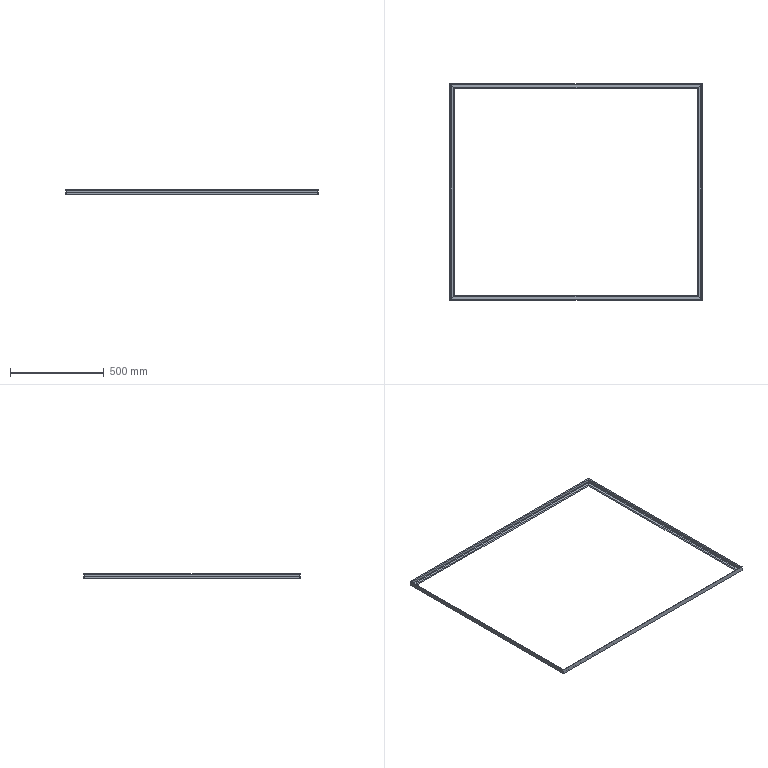Part | SolidWorks | features WeldMemberFeat 1, WeldmentFeature 1 | 4 solids | 36 faces | box 1348 x 1158 x 25 mm | volume 890268 mm3 | plane 24 | cylinder 12 | commonest cylinder face diameters 8 x8 7 x4
STEP:
#1=CARTESIAN_POINT('',(-649.,554.,0.));
#2=VERTEX_POINT('',#1);
#3=CARTESIAN_POINT('',(-674.,579.,0.));
#4=VERTEX_POINT('',#3);
#5=CARTESIAN_POINT('',(-82.5,-12.5,0.));
#6=DIRECTION('',(-0.7071,0.7071,0.));
#7=VECTOR('',#6,1000.);
#8=LINE('',#5,#7);
#9=EDGE_CURVE('',#2,#4,#8,.T.);
#10=ORIENTED_EDGE('',*,*,#9,.F.);
#11=CARTESIAN_POINT('',(-649.,-554.,0.));
#12=VERTEX_POINT('',#11);
#13=CARTESIAN_POINT('',(-649.,-579.,0.));
#14=DIRECTION('',(0.,1.,0.));
#15=VECTOR('',#14,1000.);
#16=LINE('',#13,#15);
#17=EDGE_CURVE('',#12,#2,#16,.T.);
#18=ORIENTED_EDGE('',*,*,#17,.F.);
#19=CARTESIAN_POINT('',(-674.,-579.,0.));
#20=VERTEX_POINT('',#19);
#21=CARTESIAN_POINT('',(-661.5,-566.5,0.));
#22=DIRECTION('',(0.7071,0.7071,0.));
#23=VECTOR('',#22,1000.);
#24=LINE('',#21,#23);
#25=EDGE_CURVE('',#20,#12,#24,.T.);
#26=ORIENTED_EDGE('',*,*,#25,.F.);
#27=CARTESIAN_POINT('',(-674.,-579.,0.));
#28=DIRECTION('',(0.,1.,0.));
#29=VECTOR('',#28,1000.);
#30=LINE('',#27,#29);
#31=EDGE_CURVE('',#20,#4,#30,.T.);
#32=ORIENTED_EDGE('',*,*,#31,.T.);
#33=EDGE_LOOP('',(#10,#18,#26,#32));
#34=FACE_OUTER_BOUND('',#33,.T.);
#35=CARTESIAN_POINT('',(-649.,-579.,0.));
#36=DIRECTION('',(0.,0.,1.));
#37=DIRECTION('',(1.,0.,0.));
#38=AXIS2_PLACEMENT_3D('',#35,#36,#37);
#39=PLANE('',#38);
#40=ADVANCED_FACE('',(#34),#39,.F.);
#41=CARTESIAN_POINT('',(-653.,558.,4.));
#42=VERTEX_POINT('',#41);
#43=CARTESIAN_POINT('',(-653.,558.,4.));
#44=CARTESIAN_POINT('',(-650.657,555.657,4.));
#45=CARTESIAN_POINT('',(-649.,554.,2.343));
#46=CARTESIAN_POINT('',(-649.,554.,0.));
#47=(BOUNDED_CURVE()B_SPLINE_CURVE(3,(#43,#44,#45,#46),.UNSPECIFIED.,.F.,.F.)B_SPLINE_CURVE_WITH_KNOTS((4,4),(1.571,3.142),.UNSPECIFIED.)CURVE()GEOMETRIC_REPRESENTATION_ITEM()RATIONAL_B_SPLINE_CURVE((1.,0.8047,0.8047,1.))REPRESENTATION_ITEM(''));
#48=EDGE_CURVE('',#42,#2,#47,.T.);
#49=ORIENTED_EDGE('',*,*,#48,.F.);
#50=CARTESIAN_POINT('',(-653.,-558.,4.));
#51=VERTEX_POINT('',#50);
#52=CARTESIAN_POINT('',(-653.,-579.,4.));
#53=DIRECTION('',(0.,1.,0.));
#54=VECTOR('',#53,1000.);
#55=LINE('',#52,#54);
#56=EDGE_CURVE('',#51,#42,#55,.T.);
#57=ORIENTED_EDGE('',*,*,#56,.F.);
#58=CARTESIAN_POINT('',(-649.,-554.,0.));
#59=CARTESIAN_POINT('',(-649.,-554.,2.343));
#60=CARTESIAN_POINT('',(-650.657,-555.657,4.));
#61=CARTESIAN_POINT('',(-653.,-558.,4.));
#62=(BOUNDED_CURVE()B_SPLINE_CURVE(3,(#58,#59,#60,#61),.UNSPECIFIED.,.F.,.F.)B_SPLINE_CURVE_WITH_KNOTS((4,4),(0.,1.571),.UNSPECIFIED.)CURVE()GEOMETRIC_REPRESENTATION_ITEM()RATIONAL_B_SPLINE_CURVE((1.,0.8047,0.8047,1.))REPRESENTATION_ITEM(''));
#63=EDGE_CURVE('',#12,#51,#62,.T.);
#64=ORIENTED_EDGE('',*,*,#63,.F.);
#65=ORIENTED_EDGE('',*,*,#17,.T.);
#66=EDGE_LOOP('',(#49,#57,#64,#65));
#67=FACE_OUTER_BOUND('',#66,.T.);
#68=CARTESIAN_POINT('',(-653.,-579.,0.));
#69=DIRECTION('',(0.,1.,0.));
#70=DIRECTION('',(0.,0.,1.));
#71=AXIS2_PLACEMENT_3D('',#68,#69,#70);
#72=CYLINDRICAL_SURFACE('',#71,4.);
#73=ADVANCED_FACE('',(#67),#72,.T.);
#74=CARTESIAN_POINT('',(-666.5,571.5,4.));
#75=VERTEX_POINT('',#74);
#76=CARTESIAN_POINT('',(-91.25,-3.75,4.));
#77=DIRECTION('',(0.7071,-0.7071,0.));
#78=VECTOR('',#77,1000.);
#79=LINE('',#76,#78);
#80=EDGE_CURVE('',#75,#42,#79,.T.);
#81=ORIENTED_EDGE('',*,*,#80,.F.);
#82=CARTESIAN_POINT('',(-666.5,-571.5,4.));
#83=VERTEX_POINT('',#82);
#84=CARTESIAN_POINT('',(-666.5,-579.,4.));
#85=DIRECTION('',(0.,1.,0.));
#86=VECTOR('',#85,1000.);
#87=LINE('',#84,#86);
#88=EDGE_CURVE('',#83,#75,#87,.T.);
#89=ORIENTED_EDGE('',*,*,#88,.F.);
#90=CARTESIAN_POINT('',(-670.25,-575.25,4.));
#91=DIRECTION('',(-0.7071,-0.7071,0.));
#92=VECTOR('',#91,1000.);
#93=LINE('',#90,#92);
#94=EDGE_CURVE('',#51,#83,#93,.T.);
#95=ORIENTED_EDGE('',*,*,#94,.F.);
#96=ORIENTED_EDGE('',*,*,#56,.T.);
#97=EDGE_LOOP('',(#81,#89,#95,#96));
#98=FACE_OUTER_BOUND('',#97,.T.);
#99=CARTESIAN_POINT('',(-666.5,-579.,4.));
#100=DIRECTION('',(0.,0.,-1.));
#101=DIRECTION('',(-1.,0.,0.));
#102=AXIS2_PLACEMENT_3D('',#99,#100,#101);
#103=PLANE('',#102);
#104=ADVANCED_FACE('',(#98),#103,.F.);
#105=CARTESIAN_POINT('',(-670.,575.,7.5));
#106=VERTEX_POINT('',#105);
#107=CARTESIAN_POINT('',(-670.,575.,7.5));
#108=CARTESIAN_POINT('',(-670.,575.,5.45));
#109=CARTESIAN_POINT('',(-668.55,573.55,4.));
#110=CARTESIAN_POINT('',(-666.5,571.5,4.));
#111=(BOUNDED_CURVE()B_SPLINE_CURVE(3,(#107,#108,#109,#110),.UNSPECIFIED.,.F.,.F.)B_SPLINE_CURVE_WITH_KNOTS((4,4),(0.,1.571),.UNSPECIFIED.)CURVE()GEOMETRIC_REPRESENTATION_ITEM()RATIONAL_B_SPLINE_CURVE((1.,0.8047,0.8047,1.))REPRESENTATION_ITEM(''));
#112=EDGE_CURVE('',#106,#75,#111,.T.);
#113=ORIENTED_EDGE('',*,*,#112,.F.);
#114=CARTESIAN_POINT('',(-670.,-575.,7.5));
#115=VERTEX_POINT('',#114);
#116=CARTESIAN_POINT('',(-670.,-579.,7.5));
#117=DIRECTION('',(0.,1.,0.));
#118=VECTOR('',#117,1000.);
#119=LINE('',#116,#118);
#120=EDGE_CURVE('',#115,#106,#119,.T.);
#121=ORIENTED_EDGE('',*,*,#120,.F.);
#122=CARTESIAN_POINT('',(-666.5,-571.5,4.));
#123=CARTESIAN_POINT('',(-668.55,-573.55,4.));
#124=CARTESIAN_POINT('',(-670.,-575.,5.45));
#125=CARTESIAN_POINT('',(-670.,-575.,7.5));
#126=(BOUNDED_CURVE()B_SPLINE_CURVE(3,(#122,#123,#124,#125),.UNSPECIFIED.,.F.,.F.)B_SPLINE_CURVE_WITH_KNOTS((4,4),(1.571,3.142),.UNSPECIFIED.)CURVE()GEOMETRIC_REPRESENTATION_ITEM()RATIONAL_B_SPLINE_CURVE((1.,0.8047,0.8047,1.))REPRESENTATION_ITEM(''));
#127=EDGE_CURVE('',#83,#115,#126,.T.);
#128=ORIENTED_EDGE('',*,*,#127,.F.);
#129=ORIENTED_EDGE('',*,*,#88,.T.);
#130=EDGE_LOOP('',(#113,#121,#128,#129));
#131=FACE_OUTER_BOUND('',#130,.T.);
#132=CARTESIAN_POINT('',(-666.5,-579.,7.5));
#133=DIRECTION('',(0.,1.,0.));
#134=DIRECTION('',(0.,0.,1.));
#135=AXIS2_PLACEMENT_3D('',#132,#133,#134);
#136=CYLINDRICAL_SURFACE('',#135,3.5);
#137=ADVANCED_FACE('',(#131),#136,.F.);
#138=CARTESIAN_POINT('',(-670.,575.,21.));
#139=VERTEX_POINT('',#138);
#140=CARTESIAN_POINT('',(-670.,575.,21.));
#141=DIRECTION('',(0.,0.,-1.));
#142=VECTOR('',#141,1000.);
#143=LINE('',#140,#142);
#144=EDGE_CURVE('',#139,#106,#143,.T.);
#145=ORIENTED_EDGE('',*,*,#144,.F.);
#146=CARTESIAN_POINT('',(-670.,-575.,21.));
#147=VERTEX_POINT('',#146);
#148=CARTESIAN_POINT('',(-670.,-579.,21.));
#149=DIRECTION('',(0.,1.,0.));
#150=VECTOR('',#149,1000.);
#151=LINE('',#148,#150);
#152=EDGE_CURVE('',#147,#139,#151,.T.);
#153=ORIENTED_EDGE('',*,*,#152,.F.);
#154=CARTESIAN_POINT('',(-670.,-575.,21.));
#155=DIRECTION('',(0.,0.,1.));
#156=VECTOR('',#155,1000.);
#157=LINE('',#154,#156);
#158=EDGE_CURVE('',#115,#147,#157,.T.);
#159=ORIENTED_EDGE('',*,*,#158,.F.);
#160=ORIENTED_EDGE('',*,*,#120,.T.);
#161=EDGE_LOOP('',(#145,#153,#159,#160));
#162=FACE_OUTER_BOUND('',#161,.T.);
#163=CARTESIAN_POINT('',(-670.,-579.,21.));
#164=DIRECTION('',(-1.,0.,0.));
#165=DIRECTION('',(0.,0.,1.));
#166=AXIS2_PLACEMENT_3D('',#163,#164,#165);
#167=PLANE('',#166);
#168=ADVANCED_FACE('',(#162),#167,.F.);
#169=CARTESIAN_POINT('',(-674.,579.,25.));
#170=VERTEX_POINT('',#169);
#171=CARTESIAN_POINT('',(-674.,579.,25.));
#172=CARTESIAN_POINT('',(-671.657,576.657,25.));
#173=CARTESIAN_POINT('',(-670.,575.,23.343));
#174=CARTESIAN_POINT('',(-670.,575.,21.));
#175=(BOUNDED_CURVE()B_SPLINE_CURVE(3,(#171,#172,#173,#174),.UNSPECIFIED.,.F.,.F.)B_SPLINE_CURVE_WITH_KNOTS((4,4),(1.571,3.142),.UNSPECIFIED.)CURVE()GEOMETRIC_REPRESENTATION_ITEM()RATIONAL_B_SPLINE_CURVE((1.,0.8047,0.8047,1.))REPRESENTATION_ITEM(''));
#176=EDGE_CURVE('',#170,#139,#175,.T.);
#177=ORIENTED_EDGE('',*,*,#176,.F.);
#178=CARTESIAN_POINT('',(-674.,-579.,25.));
#179=VERTEX_POINT('',#178);
#180=CARTESIAN_POINT('',(-674.,-579.,25.));
#181=DIRECTION('',(0.,1.,0.));
#182=VECTOR('',#181,1000.);
#183=LINE('',#180,#182);
#184=EDGE_CURVE('',#179,#170,#183,.T.);
#185=ORIENTED_EDGE('',*,*,#184,.F.);
#186=CARTESIAN_POINT('',(-670.,-575.,21.));
#187=CARTESIAN_POINT('',(-670.,-575.,23.343));
#188=CARTESIAN_POINT('',(-671.657,-576.657,25.));
#189=CARTESIAN_POINT('',(-674.,-579.,25.));
#190=(BOUNDED_CURVE()B_SPLINE_CURVE(3,(#186,#187,#188,#189),.UNSPECIFIED.,.F.,.F.)B_SPLINE_CURVE_WITH_KNOTS((4,4),(0.,1.571),.UNSPECIFIED.)CURVE()GEOMETRIC_REPRESENTATION_ITEM()RATIONAL_B_SPLINE_CURVE((1.,0.8047,0.8047,1.))REPRESENTATION_ITEM(''));
#191=EDGE_CURVE('',#147,#179,#190,.T.);
#192=ORIENTED_EDGE('',*,*,#191,.F.);
#193=ORIENTED_EDGE('',*,*,#152,.T.);
#194=EDGE_LOOP('',(#177,#185,#192,#193));
#195=FACE_OUTER_BOUND('',#194,.T.);
#196=CARTESIAN_POINT('',(-674.,-579.,21.));
#197=DIRECTION('',(0.,1.,0.));
#198=DIRECTION('',(0.,0.,1.));
#199=AXIS2_PLACEMENT_3D('',#196,#197,#198);
#200=CYLINDRICAL_SURFACE('',#199,4.);
#201=ADVANCED_FACE('',(#195),#200,.T.);
#202=CARTESIAN_POINT('',(-674.,579.,0.));
#203=DIRECTION('',(0.,0.,1.));
#204=VECTOR('',#203,1000.);
#205=LINE('',#202,#204);
#206=EDGE_CURVE('',#4,#170,#205,.T.);
#207=ORIENTED_EDGE('',*,*,#206,.F.);
#208=ORIENTED_EDGE('',*,*,#31,.F.);
#209=CARTESIAN_POINT('',(-674.,-579.,0.));
#210=DIRECTION('',(0.,0.,-1.));
#211=VECTOR('',#210,1000.);
#212=LINE('',#209,#211);
#213=EDGE_CURVE('',#179,#20,#212,.T.);
#214=ORIENTED_EDGE('',*,*,#213,.F.);
#215=ORIENTED_EDGE('',*,*,#184,.T.);
#216=EDGE_LOOP('',(#207,#208,#214,#215));
#217=FACE_OUTER_BOUND('',#216,.T.);
#218=CARTESIAN_POINT('',(-674.,-579.,0.));
#219=DIRECTION('',(1.,0.,0.));
#220=DIRECTION('',(0.,0.,-1.));
#221=AXIS2_PLACEMENT_3D('',#218,#219,#220);
#222=PLANE('',#221);
#223=ADVANCED_FACE('',(#217),#222,.F.);
#224=ORIENTED_EDGE('',*,*,#213,.T.);
#225=ORIENTED_EDGE('',*,*,#25,.T.);
#226=ORIENTED_EDGE('',*,*,#63,.T.);
#227=ORIENTED_EDGE('',*,*,#94,.T.);
#228=ORIENTED_EDGE('',*,*,#127,.T.);
#229=ORIENTED_EDGE('',*,*,#158,.T.);
#230=ORIENTED_EDGE('',*,*,#191,.T.);
#231=EDGE_LOOP('',(#224,#225,#226,#227,#228,#229,#230));
#232=FACE_OUTER_BOUND('',#231,.T.);
#233=CARTESIAN_POINT('',(-674.,-579.,0.));
#234=DIRECTION('',(0.7071,-0.7071,0.));
#235=DIRECTION('',(0.7071,0.7071,0.));
#236=AXIS2_PLACEMENT_3D('',#233,#234,#235);
#237=PLANE('',#236);
#238=ADVANCED_FACE('',(#232),#237,.T.);
#239=ORIENTED_EDGE('',*,*,#48,.T.);
#240=ORIENTED_EDGE('',*,*,#9,.T.);
#241=ORIENTED_EDGE('',*,*,#206,.T.);
#242=ORIENTED_EDGE('',*,*,#176,.T.);
#243=ORIENTED_EDGE('',*,*,#144,.T.);
#244=ORIENTED_EDGE('',*,*,#112,.T.);
#245=ORIENTED_EDGE('',*,*,#80,.T.);
#246=EDGE_LOOP('',(#239,#240,#241,#242,#243,#244,#245));
#247=FACE_OUTER_BOUND('',#246,.T.);
#248=CARTESIAN_POINT('',(-674.,579.,0.));
#249=DIRECTION('',(0.7071,0.7071,0.));
#250=DIRECTION('',(-0.7071,0.7071,0.));
#251=AXIS2_PLACEMENT_3D('',#248,#249,#250);
#252=PLANE('',#251);
#253=ADVANCED_FACE('',(#247),#252,.T.);
#254=CLOSED_SHELL('',(#40,#73,#104,#137,#168,#201,#223,#238,#253));
#255=MANIFOLD_SOLID_BREP('',#254);
#256=CARTESIAN_POINT('',(-649.,-554.,0.));
#257=VERTEX_POINT('',#256);
#258=CARTESIAN_POINT('',(-674.,-579.,0.));
#259=VERTEX_POINT('',#258);
#260=CARTESIAN_POINT('',(12.5,107.5,0.));
#261=DIRECTION('',(-0.7071,-0.7071,0.));
#262=VECTOR('',#261,1000.);
#263=LINE('',#260,#262);
#264=EDGE_CURVE('',#257,#259,#263,.T.);
#265=ORIENTED_EDGE('',*,*,#264,.F.);
#266=CARTESIAN_POINT('',(649.,-554.,0.));
#267=VERTEX_POINT('',#266);
#268=CARTESIAN_POINT('',(674.,-554.,0.));
#269=DIRECTION('',(-1.,0.,0.));
#270=VECTOR('',#269,1000.);
#271=LINE('',#268,#270);
#272=EDGE_CURVE('',#267,#257,#271,.T.);
#273=ORIENTED_EDGE('',*,*,#272,.F.);
#274=CARTESIAN_POINT('',(674.,-579.,0.));
#275=VERTEX_POINT('',#274);
#276=CARTESIAN_POINT('',(661.5,-566.5,0.));
#277=DIRECTION('',(-0.7071,0.7071,0.));
#278=VECTOR('',#277,1000.);
#279=LINE('',#276,#278);
#280=EDGE_CURVE('',#275,#267,#279,.T.);
#281=ORIENTED_EDGE('',*,*,#280,.F.);
#282=CARTESIAN_POINT('',(674.,-579.,0.));
#283=DIRECTION('',(-1.,0.,0.));
#284=VECTOR('',#283,1000.);
#285=LINE('',#282,#284);
#286=EDGE_CURVE('',#275,#259,#285,.T.);
#287=ORIENTED_EDGE('',*,*,#286,.T.);
#288=EDGE_LOOP('',(#265,#273,#281,#287));
#289=FACE_OUTER_BOUND('',#288,.T.);
#290=CARTESIAN_POINT('',(674.,-554.,0.));
#291=DIRECTION('',(0.,0.,1.));
#292=DIRECTION('',(1.,0.,0.));
#293=AXIS2_PLACEMENT_3D('',#290,#291,#292);
#294=PLANE('',#293);
#295=ADVANCED_FACE('',(#289),#294,.F.);
#296=CARTESIAN_POINT('',(-653.,-558.,4.));
#297=VERTEX_POINT('',#296);
#298=CARTESIAN_POINT('',(-653.,-558.,4.));
#299=CARTESIAN_POINT('',(-650.657,-555.657,4.));
#300=CARTESIAN_POINT('',(-649.,-554.,2.343));
#301=CARTESIAN_POINT('',(-649.,-554.,0.));
#302=(BOUNDED_CURVE()B_SPLINE_CURVE(3,(#298,#299,#300,#301),.UNSPECIFIED.,.F.,.T.)B_SPLINE_CURVE_WITH_KNOTS((4,4),(1.571,3.142),.UNSPECIFIED.)CURVE()GEOMETRIC_REPRESENTATION_ITEM()RATIONAL_B_SPLINE_CURVE((1.,0.8047,0.8047,1.))REPRESENTATION_ITEM(''));
#303=EDGE_CURVE('',#297,#257,#302,.T.);
#304=ORIENTED_EDGE('',*,*,#303,.F.);
#305=CARTESIAN_POINT('',(653.,-558.,4.));
#306=VERTEX_POINT('',#305);
#307=CARTESIAN_POINT('',(674.,-558.,4.));
#308=DIRECTION('',(-1.,0.,0.));
#309=VECTOR('',#308,1000.);
#310=LINE('',#307,#309);
#311=EDGE_CURVE('',#306,#297,#310,.T.);
#312=ORIENTED_EDGE('',*,*,#311,.F.);
#313=CARTESIAN_POINT('',(649.,-554.,0.));
#314=CARTESIAN_POINT('',(649.,-554.,2.343));
#315=CARTESIAN_POINT('',(650.657,-555.657,4.));
#316=CARTESIAN_POINT('',(653.,-558.,4.));
#317=(BOUNDED_CURVE()B_SPLINE_CURVE(3,(#313,#314,#315,#316),.UNSPECIFIED.,.F.,.F.)B_SPLINE_CURVE_WITH_KNOTS((4,4),(0.,1.571),.UNSPECIFIED.)CURVE()GEOMETRIC_REPRESENTATION_ITEM()RATIONAL_B_SPLINE_CURVE((1.,0.8047,0.8047,1.))REPRESENTATION_ITEM(''));
#318=EDGE_CURVE('',#267,#306,#317,.T.);
#319=ORIENTED_EDGE('',*,*,#318,.F.);
#320=ORIENTED_EDGE('',*,*,#272,.T.);
#321=EDGE_LOOP('',(#304,#312,#319,#320));
#322=FACE_OUTER_BOUND('',#321,.T.);
#323=CARTESIAN_POINT('',(674.,-558.,0.));
#324=DIRECTION('',(-1.,0.,0.));
#325=DIRECTION('',(0.,0.,1.));
#326=AXIS2_PLACEMENT_3D('',#323,#324,#325);
#327=CYLINDRICAL_SURFACE('',#326,4.);
#328=ADVANCED_FACE('',(#322),#327,.T.);
#329=CARTESIAN_POINT('',(-666.5,-571.5,4.));
#330=VERTEX_POINT('',#329);
#331=CARTESIAN_POINT('',(3.75,98.75,4.));
#332=DIRECTION('',(0.7071,0.7071,0.));
#333=VECTOR('',#332,1000.);
#334=LINE('',#331,#333);
#335=EDGE_CURVE('',#330,#297,#334,.T.);
#336=ORIENTED_EDGE('',*,*,#335,.F.);
#337=CARTESIAN_POINT('',(666.5,-571.5,4.));
#338=VERTEX_POINT('',#337);
#339=CARTESIAN_POINT('',(674.,-571.5,4.));
#340=DIRECTION('',(-1.,0.,0.));
#341=VECTOR('',#340,1000.);
#342=LINE('',#339,#341);
#343=EDGE_CURVE('',#338,#330,#342,.T.);
#344=ORIENTED_EDGE('',*,*,#343,.F.);
#345=CARTESIAN_POINT('',(670.25,-575.25,4.));
#346=DIRECTION('',(0.7071,-0.7071,0.));
#347=VECTOR('',#346,1000.);
#348=LINE('',#345,#347);
#349=EDGE_CURVE('',#306,#338,#348,.T.);
#350=ORIENTED_EDGE('',*,*,#349,.F.);
#351=ORIENTED_EDGE('',*,*,#311,.T.);
#352=EDGE_LOOP('',(#336,#344,#350,#351));
#353=FACE_OUTER_BOUND('',#352,.T.);
#354=CARTESIAN_POINT('',(674.,-571.5,4.));
#355=DIRECTION('',(0.,0.,-1.));
#356=DIRECTION('',(-1.,0.,0.));
#357=AXIS2_PLACEMENT_3D('',#354,#355,#356);
#358=PLANE('',#357);
#359=ADVANCED_FACE('',(#353),#358,.F.);
#360=CARTESIAN_POINT('',(-670.,-575.,7.5));
#361=VERTEX_POINT('',#360);
#362=CARTESIAN_POINT('',(-670.,-575.,7.5));
#363=CARTESIAN_POINT('',(-670.,-575.,5.45));
#364=CARTESIAN_POINT('',(-668.55,-573.55,4.));
#365=CARTESIAN_POINT('',(-666.5,-571.5,4.));
#366=(BOUNDED_CURVE()B_SPLINE_CURVE(3,(#362,#363,#364,#365),.UNSPECIFIED.,.F.,.T.)B_SPLINE_CURVE_WITH_KNOTS((4,4),(0.,1.571),.UNSPECIFIED.)CURVE()GEOMETRIC_REPRESENTATION_ITEM()RATIONAL_B_SPLINE_CURVE((1.,0.8047,0.8047,1.))REPRESENTATION_ITEM(''));
#367=EDGE_CURVE('',#361,#330,#366,.T.);
#368=ORIENTED_EDGE('',*,*,#367,.F.);
#369=CARTESIAN_POINT('',(670.,-575.,7.5));
#370=VERTEX_POINT('',#369);
#371=CARTESIAN_POINT('',(674.,-575.,7.5));
#372=DIRECTION('',(-1.,0.,0.));
#373=VECTOR('',#372,1000.);
#374=LINE('',#371,#373);
#375=EDGE_CURVE('',#370,#361,#374,.T.);
#376=ORIENTED_EDGE('',*,*,#375,.F.);
#377=CARTESIAN_POINT('',(666.5,-571.5,4.));
#378=CARTESIAN_POINT('',(668.55,-573.55,4.));
#379=CARTESIAN_POINT('',(670.,-575.,5.45));
#380=CARTESIAN_POINT('',(670.,-575.,7.5));
#381=(BOUNDED_CURVE()B_SPLINE_CURVE(3,(#377,#378,#379,#380),.UNSPECIFIED.,.F.,.T.)B_SPLINE_CURVE_WITH_KNOTS((4,4),(1.571,3.142),.UNSPECIFIED.)CURVE()GEOMETRIC_REPRESENTATION_ITEM()RATIONAL_B_SPLINE_CURVE((1.,0.8047,0.8047,1.))REPRESENTATION_ITEM(''));
#382=EDGE_CURVE('',#338,#370,#381,.T.);
#383=ORIENTED_EDGE('',*,*,#382,.F.);
#384=ORIENTED_EDGE('',*,*,#343,.T.);
#385=EDGE_LOOP('',(#368,#376,#383,#384));
#386=FACE_OUTER_BOUND('',#385,.T.);
#387=CARTESIAN_POINT('',(674.,-571.5,7.5));
#388=DIRECTION('',(-1.,0.,0.));
#389=DIRECTION('',(0.,0.,1.));
#390=AXIS2_PLACEMENT_3D('',#387,#388,#389);
#391=CYLINDRICAL_SURFACE('',#390,3.5);
#392=ADVANCED_FACE('',(#386),#391,.F.);
#393=CARTESIAN_POINT('',(-670.,-575.,21.));
#394=VERTEX_POINT('',#393);
#395=CARTESIAN_POINT('',(-670.,-575.,21.));
#396=DIRECTION('',(0.,0.,-1.));
#397=VECTOR('',#396,1000.);
#398=LINE('',#395,#397);
#399=EDGE_CURVE('',#394,#361,#398,.T.);
#400=ORIENTED_EDGE('',*,*,#399,.F.);
#401=CARTESIAN_POINT('',(670.,-575.,21.));
#402=VERTEX_POINT('',#401);
#403=CARTESIAN_POINT('',(674.,-575.,21.));
#404=DIRECTION('',(-1.,0.,0.));
#405=VECTOR('',#404,1000.);
#406=LINE('',#403,#405);
#407=EDGE_CURVE('',#402,#394,#406,.T.);
#408=ORIENTED_EDGE('',*,*,#407,.F.);
#409=CARTESIAN_POINT('',(670.,-575.,21.));
#410=DIRECTION('',(0.,0.,1.));
#411=VECTOR('',#410,1000.);
#412=LINE('',#409,#411);
#413=EDGE_CURVE('',#370,#402,#412,.T.);
#414=ORIENTED_EDGE('',*,*,#413,.F.);
#415=ORIENTED_EDGE('',*,*,#375,.T.);
#416=EDGE_LOOP('',(#400,#408,#414,#415));
#417=FACE_OUTER_BOUND('',#416,.T.);
#418=CARTESIAN_POINT('',(674.,-575.,21.));
#419=DIRECTION('',(0.,-1.,0.));
#420=DIRECTION('',(0.,0.,-1.));
#421=AXIS2_PLACEMENT_3D('',#418,#419,#420);
#422=PLANE('',#421);
#423=ADVANCED_FACE('',(#417),#422,.F.);
#424=CARTESIAN_POINT('',(-674.,-579.,25.));
#425=VERTEX_POINT('',#424);
#426=CARTESIAN_POINT('',(-674.,-579.,25.));
#427=CARTESIAN_POINT('',(-671.657,-576.657,25.));
#428=CARTESIAN_POINT('',(-670.,-575.,23.343));
#429=CARTESIAN_POINT('',(-670.,-575.,21.));
#430=(BOUNDED_CURVE()B_SPLINE_CURVE(3,(#426,#427,#428,#429),.UNSPECIFIED.,.F.,.T.)B_SPLINE_CURVE_WITH_KNOTS((4,4),(1.571,3.142),.UNSPECIFIED.)CURVE()GEOMETRIC_REPRESENTATION_ITEM()RATIONAL_B_SPLINE_CURVE((1.,0.8047,0.8047,1.))REPRESENTATION_ITEM(''));
#431=EDGE_CURVE('',#425,#394,#430,.T.);
#432=ORIENTED_EDGE('',*,*,#431,.F.);
#433=CARTESIAN_POINT('',(674.,-579.,25.));
#434=VERTEX_POINT('',#433);
#435=CARTESIAN_POINT('',(674.,-579.,25.));
#436=DIRECTION('',(-1.,0.,0.));
#437=VECTOR('',#436,1000.);
#438=LINE('',#435,#437);
#439=EDGE_CURVE('',#434,#425,#438,.T.);
#440=ORIENTED_EDGE('',*,*,#439,.F.);
#441=CARTESIAN_POINT('',(670.,-575.,21.));
#442=CARTESIAN_POINT('',(670.,-575.,23.343));
#443=CARTESIAN_POINT('',(671.657,-576.657,25.));
#444=CARTESIAN_POINT('',(674.,-579.,25.));
#445=(BOUNDED_CURVE()B_SPLINE_CURVE(3,(#441,#442,#443,#444),.UNSPECIFIED.,.F.,.T.)B_SPLINE_CURVE_WITH_KNOTS((4,4),(0.,1.571),.UNSPECIFIED.)CURVE()GEOMETRIC_REPRESENTATION_ITEM()RATIONAL_B_SPLINE_CURVE((1.,0.8047,0.8047,1.))REPRESENTATION_ITEM(''));
#446=EDGE_CURVE('',#402,#434,#445,.T.);
#447=ORIENTED_EDGE('',*,*,#446,.F.);
#448=ORIENTED_EDGE('',*,*,#407,.T.);
#449=EDGE_LOOP('',(#432,#440,#447,#448));
#450=FACE_OUTER_BOUND('',#449,.T.);
#451=CARTESIAN_POINT('',(674.,-579.,21.));
#452=DIRECTION('',(-1.,0.,0.));
#453=DIRECTION('',(0.,0.,1.));
#454=AXIS2_PLACEMENT_3D('',#451,#452,#453);
#455=CYLINDRICAL_SURFACE('',#454,4.);
#456=ADVANCED_FACE('',(#450),#455,.T.);
#457=CARTESIAN_POINT('',(-674.,-579.,0.));
#458=DIRECTION('',(0.,0.,1.));
#459=VECTOR('',#458,1000.);
#460=LINE('',#457,#459);
#461=EDGE_CURVE('',#259,#425,#460,.T.);
#462=ORIENTED_EDGE('',*,*,#461,.F.);
#463=ORIENTED_EDGE('',*,*,#286,.F.);
#464=CARTESIAN_POINT('',(674.,-579.,0.));
#465=DIRECTION('',(0.,0.,-1.));
#466=VECTOR('',#465,1000.);
#467=LINE('',#464,#466);
#468=EDGE_CURVE('',#434,#275,#467,.T.);
#469=ORIENTED_EDGE('',*,*,#468,.F.);
#470=ORIENTED_EDGE('',*,*,#439,.T.);
#471=EDGE_LOOP('',(#462,#463,#469,#470));
#472=FACE_OUTER_BOUND('',#471,.T.);
#473=CARTESIAN_POINT('',(674.,-579.,0.));
#474=DIRECTION('',(0.,1.,0.));
#475=DIRECTION('',(0.,0.,1.));
#476=AXIS2_PLACEMENT_3D('',#473,#474,#475);
#477=PLANE('',#476);
#478=ADVANCED_FACE('',(#472),#477,.F.);
#479=ORIENTED_EDGE('',*,*,#468,.T.);
#480=ORIENTED_EDGE('',*,*,#280,.T.);
#481=ORIENTED_EDGE('',*,*,#318,.T.);
#482=ORIENTED_EDGE('',*,*,#349,.T.);
#483=ORIENTED_EDGE('',*,*,#382,.T.);
#484=ORIENTED_EDGE('',*,*,#413,.T.);
#485=ORIENTED_EDGE('',*,*,#446,.T.);
#486=EDGE_LOOP('',(#479,#480,#481,#482,#483,#484,#485));
#487=FACE_OUTER_BOUND('',#486,.T.);
#488=CARTESIAN_POINT('',(674.,-579.,0.));
#489=DIRECTION('',(0.7071,0.7071,0.));
#490=DIRECTION('',(-0.7071,0.7071,0.));
#491=AXIS2_PLACEMENT_3D('',#488,#489,#490);
#492=PLANE('',#491);
#493=ADVANCED_FACE('',(#487),#492,.T.);
#494=ORIENTED_EDGE('',*,*,#303,.T.);
#495=ORIENTED_EDGE('',*,*,#264,.T.);
#496=ORIENTED_EDGE('',*,*,#461,.T.);
#497=ORIENTED_EDGE('',*,*,#431,.T.);
#498=ORIENTED_EDGE('',*,*,#399,.T.);
#499=ORIENTED_EDGE('',*,*,#367,.T.);
#500=ORIENTED_EDGE('',*,*,#335,.T.);
#501=EDGE_LOOP('',(#494,#495,#496,#497,#498,#499,#500));
#502=FACE_OUTER_BOUND('',#501,.T.);
#503=CARTESIAN_POINT('',(-674.,-579.,0.));
#504=DIRECTION('',(-0.7071,0.7071,0.));
#505=DIRECTION('',(-0.7071,-0.7071,0.));
#506=AXIS2_PLACEMENT_3D('',#503,#504,#505);
#507=PLANE('',#506);
#508=ADVANCED_FACE('',(#502),#507,.T.);
#509=CLOSED_SHELL('',(#295,#328,#359,#392,#423,#456,#478,#493,#508));
#510=MANIFOLD_SOLID_BREP('',#509);
#511=CARTESIAN_POINT('',(649.,-554.,0.));
#512=VERTEX_POINT('',#511);
#513=CARTESIAN_POINT('',(674.,-579.,0.));
#514=VERTEX_POINT('',#513);
#515=CARTESIAN_POINT('',(82.5,12.5,0.));
#516=DIRECTION('',(0.7071,-0.7071,0.));
#517=VECTOR('',#516,1000.);
#518=LINE('',#515,#517);
#519=EDGE_CURVE('',#512,#514,#518,.T.);
#520=ORIENTED_EDGE('',*,*,#519,.F.);
#521=CARTESIAN_POINT('',(649.,554.,0.));
#522=VERTEX_POINT('',#521);
#523=CARTESIAN_POINT('',(649.,579.,0.));
#524=DIRECTION('',(0.,-1.,0.));
#525=VECTOR('',#524,1000.);
#526=LINE('',#523,#525);
#527=EDGE_CURVE('',#522,#512,#526,.T.);
#528=ORIENTED_EDGE('',*,*,#527,.F.);
#529=CARTESIAN_POINT('',(674.,579.,0.));
#530=VERTEX_POINT('',#529);
#531=CARTESIAN_POINT('',(661.5,566.5,0.));
#532=DIRECTION('',(-0.7071,-0.7071,0.));
#533=VECTOR('',#532,1000.);
#534=LINE('',#531,#533);
#535=EDGE_CURVE('',#530,#522,#534,.T.);
#536=ORIENTED_EDGE('',*,*,#535,.F.);
#537=CARTESIAN_POINT('',(674.,579.,0.));
#538=DIRECTION('',(0.,-1.,0.));
#539=VECTOR('',#538,1000.);
#540=LINE('',#537,#539);
#541=EDGE_CURVE('',#530,#514,#540,.T.);
#542=ORIENTED_EDGE('',*,*,#541,.T.);
#543=EDGE_LOOP('',(#520,#528,#536,#542));
#544=FACE_OUTER_BOUND('',#543,.T.);
#545=CARTESIAN_POINT('',(649.,579.,0.));
#546=DIRECTION('',(0.,0.,1.));
#547=DIRECTION('',(1.,0.,0.));
#548=AXIS2_PLACEMENT_3D('',#545,#546,#547);
#549=PLANE('',#548);
#550=ADVANCED_FACE('',(#544),#549,.F.);
#551=CARTESIAN_POINT('',(653.,-558.,4.));
#552=VERTEX_POINT('',#551);
#553=CARTESIAN_POINT('',(653.,-558.,4.));
#554=CARTESIAN_POINT('',(650.657,-555.657,4.));
#555=CARTESIAN_POINT('',(649.,-554.,2.343));
#556=CARTESIAN_POINT('',(649.,-554.,0.));
#557=(BOUNDED_CURVE()B_SPLINE_CURVE(3,(#553,#554,#555,#556),.UNSPECIFIED.,.F.,.F.)B_SPLINE_CURVE_WITH_KNOTS((4,4),(1.571,3.142),.UNSPECIFIED.)CURVE()GEOMETRIC_REPRESENTATION_ITEM()RATIONAL_B_SPLINE_CURVE((1.,0.8047,0.8047,1.))REPRESENTATION_ITEM(''));
#558=EDGE_CURVE('',#552,#512,#557,.T.);
#559=ORIENTED_EDGE('',*,*,#558,.F.);
#560=CARTESIAN_POINT('',(653.,558.,4.));
#561=VERTEX_POINT('',#560);
#562=CARTESIAN_POINT('',(653.,579.,4.));
#563=DIRECTION('',(0.,-1.,0.));
#564=VECTOR('',#563,1000.);
#565=LINE('',#562,#564);
#566=EDGE_CURVE('',#561,#552,#565,.T.);
#567=ORIENTED_EDGE('',*,*,#566,.F.);
#568=CARTESIAN_POINT('',(649.,554.,0.));
#569=CARTESIAN_POINT('',(649.,554.,2.343));
#570=CARTESIAN_POINT('',(650.657,555.657,4.));
#571=CARTESIAN_POINT('',(653.,558.,4.));
#572=(BOUNDED_CURVE()B_SPLINE_CURVE(3,(#568,#569,#570,#571),.UNSPECIFIED.,.F.,.F.)B_SPLINE_CURVE_WITH_KNOTS((4,4),(0.,1.571),.UNSPECIFIED.)CURVE()GEOMETRIC_REPRESENTATION_ITEM()RATIONAL_B_SPLINE_CURVE((1.,0.8047,0.8047,1.))REPRESENTATION_ITEM(''));
#573=EDGE_CURVE('',#522,#561,#572,.T.);
#574=ORIENTED_EDGE('',*,*,#573,.F.);
#575=ORIENTED_EDGE('',*,*,#527,.T.);
#576=EDGE_LOOP('',(#559,#567,#574,#575));
#577=FACE_OUTER_BOUND('',#576,.T.);
#578=CARTESIAN_POINT('',(653.,579.,0.));
#579=DIRECTION('',(0.,-1.,0.));
#580=DIRECTION('',(0.,0.,-1.));
#581=AXIS2_PLACEMENT_3D('',#578,#579,#580);
#582=CYLINDRICAL_SURFACE('',#581,4.);
#583=ADVANCED_FACE('',(#577),#582,.T.);
#584=CARTESIAN_POINT('',(666.5,-571.5,4.));
#585=VERTEX_POINT('',#584);
#586=CARTESIAN_POINT('',(91.25,3.75,4.));
#587=DIRECTION('',(-0.7071,0.7071,0.));
#588=VECTOR('',#587,1000.);
#589=LINE('',#586,#588);
#590=EDGE_CURVE('',#585,#552,#589,.T.);
#591=ORIENTED_EDGE('',*,*,#590,.F.);
#592=CARTESIAN_POINT('',(666.5,571.5,4.));
#593=VERTEX_POINT('',#592);
#594=CARTESIAN_POINT('',(666.5,579.,4.));
#595=DIRECTION('',(0.,-1.,0.));
#596=VECTOR('',#595,1000.);
#597=LINE('',#594,#596);
#598=EDGE_CURVE('',#593,#585,#597,.T.);
#599=ORIENTED_EDGE('',*,*,#598,.F.);
#600=CARTESIAN_POINT('',(670.25,575.25,4.));
#601=DIRECTION('',(0.7071,0.7071,0.));
#602=VECTOR('',#601,1000.);
#603=LINE('',#600,#602);
#604=EDGE_CURVE('',#561,#593,#603,.T.);
#605=ORIENTED_EDGE('',*,*,#604,.F.);
#606=ORIENTED_EDGE('',*,*,#566,.T.);
#607=EDGE_LOOP('',(#591,#599,#605,#606));
#608=FACE_OUTER_BOUND('',#607,.T.);
#609=CARTESIAN_POINT('',(666.5,579.,4.));
#610=DIRECTION('',(0.,0.,-1.));
#611=DIRECTION('',(-1.,0.,0.));
#612=AXIS2_PLACEMENT_3D('',#609,#610,#611);
#613=PLANE('',#612);
#614=ADVANCED_FACE('',(#608),#613,.F.);
#615=CARTESIAN_POINT('',(670.,-575.,7.5));
#616=VERTEX_POINT('',#615);
#617=CARTESIAN_POINT('',(670.,-575.,7.5));
#618=CARTESIAN_POINT('',(670.,-575.,5.45));
#619=CARTESIAN_POINT('',(668.55,-573.55,4.));
#620=CARTESIAN_POINT('',(666.5,-571.5,4.));
#621=(BOUNDED_CURVE()B_SPLINE_CURVE(3,(#617,#618,#619,#620),.UNSPECIFIED.,.F.,.F.)B_SPLINE_CURVE_WITH_KNOTS((4,4),(0.,1.571),.UNSPECIFIED.)CURVE()GEOMETRIC_REPRESENTATION_ITEM()RATIONAL_B_SPLINE_CURVE((1.,0.8047,0.8047,1.))REPRESENTATION_ITEM(''));
#622=EDGE_CURVE('',#616,#585,#621,.T.);
#623=ORIENTED_EDGE('',*,*,#622,.F.);
#624=CARTESIAN_POINT('',(670.,575.,7.5));
#625=VERTEX_POINT('',#624);
#626=CARTESIAN_POINT('',(670.,579.,7.5));
#627=DIRECTION('',(0.,-1.,0.));
#628=VECTOR('',#627,1000.);
#629=LINE('',#626,#628);
#630=EDGE_CURVE('',#625,#616,#629,.T.);
#631=ORIENTED_EDGE('',*,*,#630,.F.);
#632=CARTESIAN_POINT('',(666.5,571.5,4.));
#633=CARTESIAN_POINT('',(668.55,573.55,4.));
#634=CARTESIAN_POINT('',(670.,575.,5.45));
#635=CARTESIAN_POINT('',(670.,575.,7.5));
#636=(BOUNDED_CURVE()B_SPLINE_CURVE(3,(#632,#633,#634,#635),.UNSPECIFIED.,.F.,.T.)B_SPLINE_CURVE_WITH_KNOTS((4,4),(1.571,3.142),.UNSPECIFIED.)CURVE()GEOMETRIC_REPRESENTATION_ITEM()RATIONAL_B_SPLINE_CURVE((1.,0.8047,0.8047,1.))REPRESENTATION_ITEM(''));
#637=EDGE_CURVE('',#593,#625,#636,.T.);
#638=ORIENTED_EDGE('',*,*,#637,.F.);
#639=ORIENTED_EDGE('',*,*,#598,.T.);
#640=EDGE_LOOP('',(#623,#631,#638,#639));
#641=FACE_OUTER_BOUND('',#640,.T.);
#642=CARTESIAN_POINT('',(666.5,579.,7.5));
#643=DIRECTION('',(0.,-1.,0.));
#644=DIRECTION('',(0.,0.,-1.));
#645=AXIS2_PLACEMENT_3D('',#642,#643,#644);
#646=CYLINDRICAL_SURFACE('',#645,3.5);
#647=ADVANCED_FACE('',(#641),#646,.F.);
#648=CARTESIAN_POINT('',(670.,-575.,21.));
#649=VERTEX_POINT('',#648);
#650=CARTESIAN_POINT('',(670.,-575.,21.));
#651=DIRECTION('',(0.,0.,-1.));
#652=VECTOR('',#651,1000.);
#653=LINE('',#650,#652);
#654=EDGE_CURVE('',#649,#616,#653,.T.);
#655=ORIENTED_EDGE('',*,*,#654,.F.);
#656=CARTESIAN_POINT('',(670.,575.,21.));
#657=VERTEX_POINT('',#656);
#658=CARTESIAN_POINT('',(670.,579.,21.));
#659=DIRECTION('',(0.,-1.,0.));
#660=VECTOR('',#659,1000.);
#661=LINE('',#658,#660);
#662=EDGE_CURVE('',#657,#649,#661,.T.);
#663=ORIENTED_EDGE('',*,*,#662,.F.);
#664=CARTESIAN_POINT('',(670.,575.,21.));
#665=DIRECTION('',(0.,0.,1.));
#666=VECTOR('',#665,1000.);
#667=LINE('',#664,#666);
#668=EDGE_CURVE('',#625,#657,#667,.T.);
#669=ORIENTED_EDGE('',*,*,#668,.F.);
#670=ORIENTED_EDGE('',*,*,#630,.T.);
#671=EDGE_LOOP('',(#655,#663,#669,#670));
#672=FACE_OUTER_BOUND('',#671,.T.);
#673=CARTESIAN_POINT('',(670.,579.,21.));
#674=DIRECTION('',(1.,0.,0.));
#675=DIRECTION('',(0.,0.,-1.));
#676=AXIS2_PLACEMENT_3D('',#673,#674,#675);
#677=PLANE('',#676);
#678=ADVANCED_FACE('',(#672),#677,.F.);
#679=CARTESIAN_POINT('',(674.,-579.,25.));
#680=VERTEX_POINT('',#679);
#681=CARTESIAN_POINT('',(674.,-579.,25.));
#682=CARTESIAN_POINT('',(671.657,-576.657,25.));
#683=CARTESIAN_POINT('',(670.,-575.,23.343));
#684=CARTESIAN_POINT('',(670.,-575.,21.));
#685=(BOUNDED_CURVE()B_SPLINE_CURVE(3,(#681,#682,#683,#684),.UNSPECIFIED.,.F.,.F.)B_SPLINE_CURVE_WITH_KNOTS((4,4),(1.571,3.142),.UNSPECIFIED.)CURVE()GEOMETRIC_REPRESENTATION_ITEM()RATIONAL_B_SPLINE_CURVE((1.,0.8047,0.8047,1.))REPRESENTATION_ITEM(''));
#686=EDGE_CURVE('',#680,#649,#685,.T.);
#687=ORIENTED_EDGE('',*,*,#686,.F.);
#688=CARTESIAN_POINT('',(674.,579.,25.));
#689=VERTEX_POINT('',#688);
#690=CARTESIAN_POINT('',(674.,579.,25.));
#691=DIRECTION('',(0.,-1.,0.));
#692=VECTOR('',#691,1000.);
#693=LINE('',#690,#692);
#694=EDGE_CURVE('',#689,#680,#693,.T.);
#695=ORIENTED_EDGE('',*,*,#694,.F.);
#696=CARTESIAN_POINT('',(670.,575.,21.));
#697=CARTESIAN_POINT('',(670.,575.,23.343));
#698=CARTESIAN_POINT('',(671.657,576.657,25.));
#699=CARTESIAN_POINT('',(674.,579.,25.));
#700=(BOUNDED_CURVE()B_SPLINE_CURVE(3,(#696,#697,#698,#699),.UNSPECIFIED.,.F.,.T.)B_SPLINE_CURVE_WITH_KNOTS((4,4),(0.,1.571),.UNSPECIFIED.)CURVE()GEOMETRIC_REPRESENTATION_ITEM()RATIONAL_B_SPLINE_CURVE((1.,0.8047,0.8047,1.))REPRESENTATION_ITEM(''));
#701=EDGE_CURVE('',#657,#689,#700,.T.);
#702=ORIENTED_EDGE('',*,*,#701,.F.);
#703=ORIENTED_EDGE('',*,*,#662,.T.);
#704=EDGE_LOOP('',(#687,#695,#702,#703));
#705=FACE_OUTER_BOUND('',#704,.T.);
#706=CARTESIAN_POINT('',(674.,579.,21.));
#707=DIRECTION('',(0.,-1.,0.));
#708=DIRECTION('',(0.,0.,-1.));
#709=AXIS2_PLACEMENT_3D('',#706,#707,#708);
#710=CYLINDRICAL_SURFACE('',#709,4.);
#711=ADVANCED_FACE('',(#705),#710,.T.);
#712=CARTESIAN_POINT('',(674.,-579.,0.));
#713=DIRECTION('',(0.,0.,1.));
#714=VECTOR('',#713,1000.);
#715=LINE('',#712,#714);
#716=EDGE_CURVE('',#514,#680,#715,.T.);
#717=ORIENTED_EDGE('',*,*,#716,.F.);
#718=ORIENTED_EDGE('',*,*,#541,.F.);
#719=CARTESIAN_POINT('',(674.,579.,0.));
#720=DIRECTION('',(0.,0.,-1.));
#721=VECTOR('',#720,1000.);
#722=LINE('',#719,#721);
#723=EDGE_CURVE('',#689,#530,#722,.T.);
#724=ORIENTED_EDGE('',*,*,#723,.F.);
#725=ORIENTED_EDGE('',*,*,#694,.T.);
#726=EDGE_LOOP('',(#717,#718,#724,#725));
#727=FACE_OUTER_BOUND('',#726,.T.);
#728=CARTESIAN_POINT('',(674.,579.,0.));
#729=DIRECTION('',(-1.,0.,0.));
#730=DIRECTION('',(0.,0.,1.));
#731=AXIS2_PLACEMENT_3D('',#728,#729,#730);
#732=PLANE('',#731);
#733=ADVANCED_FACE('',(#727),#732,.F.);
#734=ORIENTED_EDGE('',*,*,#723,.T.);
#735=ORIENTED_EDGE('',*,*,#535,.T.);
#736=ORIENTED_EDGE('',*,*,#573,.T.);
#737=ORIENTED_EDGE('',*,*,#604,.T.);
#738=ORIENTED_EDGE('',*,*,#637,.T.);
#739=ORIENTED_EDGE('',*,*,#668,.T.);
#740=ORIENTED_EDGE('',*,*,#701,.T.);
#741=EDGE_LOOP('',(#734,#735,#736,#737,#738,#739,#740));
#742=FACE_OUTER_BOUND('',#741,.T.);
#743=CARTESIAN_POINT('',(674.,579.,0.));
#744=DIRECTION('',(-0.7071,0.7071,0.));
#745=DIRECTION('',(-0.7071,-0.7071,0.));
#746=AXIS2_PLACEMENT_3D('',#743,#744,#745);
#747=PLANE('',#746);
#748=ADVANCED_FACE('',(#742),#747,.T.);
#749=ORIENTED_EDGE('',*,*,#558,.T.);
#750=ORIENTED_EDGE('',*,*,#519,.T.);
#751=ORIENTED_EDGE('',*,*,#716,.T.);
#752=ORIENTED_EDGE('',*,*,#686,.T.);
#753=ORIENTED_EDGE('',*,*,#654,.T.);
#754=ORIENTED_EDGE('',*,*,#622,.T.);
#755=ORIENTED_EDGE('',*,*,#590,.T.);
#756=EDGE_LOOP('',(#749,#750,#751,#752,#753,#754,#755));
#757=FACE_OUTER_BOUND('',#756,.T.);
#758=CARTESIAN_POINT('',(674.,-579.,0.));
#759=DIRECTION('',(-0.7071,-0.7071,0.));
#760=DIRECTION('',(0.7071,-0.7071,0.));
#761=AXIS2_PLACEMENT_3D('',#758,#759,#760);
#762=PLANE('',#761);
#763=ADVANCED_FACE('',(#757),#762,.T.);
#764=CLOSED_SHELL('',(#550,#583,#614,#647,#678,#711,#733,#748,#763));
#765=MANIFOLD_SOLID_BREP('',#764);
#766=CARTESIAN_POINT('',(-674.,579.,0.));
#767=VERTEX_POINT('',#766);
#768=CARTESIAN_POINT('',(-649.,554.,0.));
#769=VERTEX_POINT('',#768);
#770=CARTESIAN_POINT('',(-661.5,566.5,0.));
#771=DIRECTION('',(0.7071,-0.7071,0.));
#772=VECTOR('',#771,1000.);
#773=LINE('',#770,#772);
#774=EDGE_CURVE('',#767,#769,#773,.T.);
#775=ORIENTED_EDGE('',*,*,#774,.F.);
#776=CARTESIAN_POINT('',(674.,579.,0.));
#777=VERTEX_POINT('',#776);
#778=CARTESIAN_POINT('',(-674.,579.,0.));
#779=DIRECTION('',(1.,0.,0.));
#780=VECTOR('',#779,1000.);
#781=LINE('',#778,#780);
#782=EDGE_CURVE('',#767,#777,#781,.T.);
#783=ORIENTED_EDGE('',*,*,#782,.T.);
#784=CARTESIAN_POINT('',(649.,554.,0.));
#785=VERTEX_POINT('',#784);
#786=CARTESIAN_POINT('',(-12.5,-107.5,0.));
#787=DIRECTION('',(0.7071,0.7071,0.));
#788=VECTOR('',#787,1000.);
#789=LINE('',#786,#788);
#790=EDGE_CURVE('',#785,#777,#789,.T.);
#791=ORIENTED_EDGE('',*,*,#790,.F.);
#792=CARTESIAN_POINT('',(-674.,554.,0.));
#793=DIRECTION('',(1.,0.,0.));
#794=VECTOR('',#793,1000.);
#795=LINE('',#792,#794);
#796=EDGE_CURVE('',#769,#785,#795,.T.);
#797=ORIENTED_EDGE('',*,*,#796,.F.);
#798=EDGE_LOOP('',(#775,#783,#791,#797));
#799=FACE_OUTER_BOUND('',#798,.T.);
#800=CARTESIAN_POINT('',(-674.,554.,0.));
#801=DIRECTION('',(0.,0.,1.));
#802=DIRECTION('',(1.,0.,0.));
#803=AXIS2_PLACEMENT_3D('',#800,#801,#802);
#804=PLANE('',#803);
#805=ADVANCED_FACE('',(#799),#804,.F.);
#806=CARTESIAN_POINT('',(-653.,558.,4.));
#807=VERTEX_POINT('',#806);
#808=CARTESIAN_POINT('',(-649.,554.,0.));
#809=CARTESIAN_POINT('',(-649.,554.,2.343));
#810=CARTESIAN_POINT('',(-650.657,555.657,4.));
#811=CARTESIAN_POINT('',(-653.,558.,4.));
#812=(BOUNDED_CURVE()B_SPLINE_CURVE(3,(#808,#809,#810,#811),.UNSPECIFIED.,.F.,.T.)B_SPLINE_CURVE_WITH_KNOTS((4,4),(0.,1.571),.UNSPECIFIED.)CURVE()GEOMETRIC_REPRESENTATION_ITEM()RATIONAL_B_SPLINE_CURVE((1.,0.8047,0.8047,1.))REPRESENTATION_ITEM(''));
#813=EDGE_CURVE('',#769,#807,#812,.T.);
#814=ORIENTED_EDGE('',*,*,#813,.F.);
#815=ORIENTED_EDGE('',*,*,#796,.T.);
#816=CARTESIAN_POINT('',(653.,558.,4.));
#817=VERTEX_POINT('',#816);
#818=CARTESIAN_POINT('',(653.,558.,4.));
#819=CARTESIAN_POINT('',(650.657,555.657,4.));
#820=CARTESIAN_POINT('',(649.,554.,2.343));
#821=CARTESIAN_POINT('',(649.,554.,0.));
#822=(BOUNDED_CURVE()B_SPLINE_CURVE(3,(#818,#819,#820,#821),.UNSPECIFIED.,.F.,.F.)B_SPLINE_CURVE_WITH_KNOTS((4,4),(1.571,3.142),.UNSPECIFIED.)CURVE()GEOMETRIC_REPRESENTATION_ITEM()RATIONAL_B_SPLINE_CURVE((1.,0.8047,0.8047,1.))REPRESENTATION_ITEM(''));
#823=EDGE_CURVE('',#817,#785,#822,.T.);
#824=ORIENTED_EDGE('',*,*,#823,.F.);
#825=CARTESIAN_POINT('',(-674.,558.,4.));
#826=DIRECTION('',(1.,0.,0.));
#827=VECTOR('',#826,1000.);
#828=LINE('',#825,#827);
#829=EDGE_CURVE('',#807,#817,#828,.T.);
#830=ORIENTED_EDGE('',*,*,#829,.F.);
#831=EDGE_LOOP('',(#814,#815,#824,#830));
#832=FACE_OUTER_BOUND('',#831,.T.);
#833=CARTESIAN_POINT('',(-674.,558.,0.));
#834=DIRECTION('',(1.,0.,0.));
#835=DIRECTION('',(0.,0.,-1.));
#836=AXIS2_PLACEMENT_3D('',#833,#834,#835);
#837=CYLINDRICAL_SURFACE('',#836,4.);
#838=ADVANCED_FACE('',(#832),#837,.T.);
#839=CARTESIAN_POINT('',(-666.5,571.5,4.));
#840=VERTEX_POINT('',#839);
#841=CARTESIAN_POINT('',(-670.25,575.25,4.));
#842=DIRECTION('',(-0.7071,0.7071,0.));
#843=VECTOR('',#842,1000.);
#844=LINE('',#841,#843);
#845=EDGE_CURVE('',#807,#840,#844,.T.);
#846=ORIENTED_EDGE('',*,*,#845,.F.);
#847=ORIENTED_EDGE('',*,*,#829,.T.);
#848=CARTESIAN_POINT('',(666.5,571.5,4.));
#849=VERTEX_POINT('',#848);
#850=CARTESIAN_POINT('',(-3.75,-98.75,4.));
#851=DIRECTION('',(-0.7071,-0.7071,0.));
#852=VECTOR('',#851,1000.);
#853=LINE('',#850,#852);
#854=EDGE_CURVE('',#849,#817,#853,.T.);
#855=ORIENTED_EDGE('',*,*,#854,.F.);
#856=CARTESIAN_POINT('',(-674.,571.5,4.));
#857=DIRECTION('',(1.,0.,0.));
#858=VECTOR('',#857,1000.);
#859=LINE('',#856,#858);
#860=EDGE_CURVE('',#840,#849,#859,.T.);
#861=ORIENTED_EDGE('',*,*,#860,.F.);
#862=EDGE_LOOP('',(#846,#847,#855,#861));
#863=FACE_OUTER_BOUND('',#862,.T.);
#864=CARTESIAN_POINT('',(-674.,571.5,4.));
#865=DIRECTION('',(0.,0.,-1.));
#866=DIRECTION('',(-1.,0.,0.));
#867=AXIS2_PLACEMENT_3D('',#864,#865,#866);
#868=PLANE('',#867);
#869=ADVANCED_FACE('',(#863),#868,.F.);
#870=CARTESIAN_POINT('',(-670.,575.,7.5));
#871=VERTEX_POINT('',#870);
#872=CARTESIAN_POINT('',(-666.5,571.5,4.));
#873=CARTESIAN_POINT('',(-668.55,573.55,4.));
#874=CARTESIAN_POINT('',(-670.,575.,5.45));
#875=CARTESIAN_POINT('',(-670.,575.,7.5));
#876=(BOUNDED_CURVE()B_SPLINE_CURVE(3,(#872,#873,#874,#875),.UNSPECIFIED.,.F.,.F.)B_SPLINE_CURVE_WITH_KNOTS((4,4),(1.571,3.142),.UNSPECIFIED.)CURVE()GEOMETRIC_REPRESENTATION_ITEM()RATIONAL_B_SPLINE_CURVE((1.,0.8047,0.8047,1.))REPRESENTATION_ITEM(''));
#877=EDGE_CURVE('',#840,#871,#876,.T.);
#878=ORIENTED_EDGE('',*,*,#877,.F.);
#879=ORIENTED_EDGE('',*,*,#860,.T.);
#880=CARTESIAN_POINT('',(670.,575.,7.5));
#881=VERTEX_POINT('',#880);
#882=CARTESIAN_POINT('',(670.,575.,7.5));
#883=CARTESIAN_POINT('',(670.,575.,5.45));
#884=CARTESIAN_POINT('',(668.55,573.55,4.));
#885=CARTESIAN_POINT('',(666.5,571.5,4.));
#886=(BOUNDED_CURVE()B_SPLINE_CURVE(3,(#882,#883,#884,#885),.UNSPECIFIED.,.F.,.T.)B_SPLINE_CURVE_WITH_KNOTS((4,4),(0.,1.571),.UNSPECIFIED.)CURVE()GEOMETRIC_REPRESENTATION_ITEM()RATIONAL_B_SPLINE_CURVE((1.,0.8047,0.8047,1.))REPRESENTATION_ITEM(''));
#887=EDGE_CURVE('',#881,#849,#886,.T.);
#888=ORIENTED_EDGE('',*,*,#887,.F.);
#889=CARTESIAN_POINT('',(-674.,575.,7.5));
#890=DIRECTION('',(1.,0.,0.));
#891=VECTOR('',#890,1000.);
#892=LINE('',#889,#891);
#893=EDGE_CURVE('',#871,#881,#892,.T.);
#894=ORIENTED_EDGE('',*,*,#893,.F.);
#895=EDGE_LOOP('',(#878,#879,#888,#894));
#896=FACE_OUTER_BOUND('',#895,.T.);
#897=CARTESIAN_POINT('',(-674.,571.5,7.5));
#898=DIRECTION('',(1.,0.,0.));
#899=DIRECTION('',(0.,0.,-1.));
#900=AXIS2_PLACEMENT_3D('',#897,#898,#899);
#901=CYLINDRICAL_SURFACE('',#900,3.5);
#902=ADVANCED_FACE('',(#896),#901,.F.);
#903=CARTESIAN_POINT('',(-670.,575.,21.));
#904=VERTEX_POINT('',#903);
#905=CARTESIAN_POINT('',(-670.,575.,21.));
#906=DIRECTION('',(0.,0.,1.));
#907=VECTOR('',#906,1000.);
#908=LINE('',#905,#907);
#909=EDGE_CURVE('',#871,#904,#908,.T.);
#910=ORIENTED_EDGE('',*,*,#909,.F.);
#911=ORIENTED_EDGE('',*,*,#893,.T.);
#912=CARTESIAN_POINT('',(670.,575.,21.));
#913=VERTEX_POINT('',#912);
#914=CARTESIAN_POINT('',(670.,575.,21.));
#915=DIRECTION('',(0.,0.,-1.));
#916=VECTOR('',#915,1000.);
#917=LINE('',#914,#916);
#918=EDGE_CURVE('',#913,#881,#917,.T.);
#919=ORIENTED_EDGE('',*,*,#918,.F.);
#920=CARTESIAN_POINT('',(-674.,575.,21.));
#921=DIRECTION('',(1.,0.,0.));
#922=VECTOR('',#921,1000.);
#923=LINE('',#920,#922);
#924=EDGE_CURVE('',#904,#913,#923,.T.);
#925=ORIENTED_EDGE('',*,*,#924,.F.);
#926=EDGE_LOOP('',(#910,#911,#919,#925));
#927=FACE_OUTER_BOUND('',#926,.T.);
#928=CARTESIAN_POINT('',(-674.,575.,21.));
#929=DIRECTION('',(0.,1.,0.));
#930=DIRECTION('',(0.,0.,1.));
#931=AXIS2_PLACEMENT_3D('',#928,#929,#930);
#932=PLANE('',#931);
#933=ADVANCED_FACE('',(#927),#932,.F.);
#934=CARTESIAN_POINT('',(-674.,579.,25.));
#935=VERTEX_POINT('',#934);
#936=CARTESIAN_POINT('',(-670.,575.,21.));
#937=CARTESIAN_POINT('',(-670.,575.,23.343));
#938=CARTESIAN_POINT('',(-671.657,576.657,25.));
#939=CARTESIAN_POINT('',(-674.,579.,25.));
#940=(BOUNDED_CURVE()B_SPLINE_CURVE(3,(#936,#937,#938,#939),.UNSPECIFIED.,.F.,.F.)B_SPLINE_CURVE_WITH_KNOTS((4,4),(0.,1.571),.UNSPECIFIED.)CURVE()GEOMETRIC_REPRESENTATION_ITEM()RATIONAL_B_SPLINE_CURVE((1.,0.8047,0.8047,1.))REPRESENTATION_ITEM(''));
#941=EDGE_CURVE('',#904,#935,#940,.T.);
#942=ORIENTED_EDGE('',*,*,#941,.F.);
#943=ORIENTED_EDGE('',*,*,#924,.T.);
#944=CARTESIAN_POINT('',(674.,579.,25.));
#945=VERTEX_POINT('',#944);
#946=CARTESIAN_POINT('',(674.,579.,25.));
#947=CARTESIAN_POINT('',(671.657,576.657,25.));
#948=CARTESIAN_POINT('',(670.,575.,23.343));
#949=CARTESIAN_POINT('',(670.,575.,21.));
#950=(BOUNDED_CURVE()B_SPLINE_CURVE(3,(#946,#947,#948,#949),.UNSPECIFIED.,.F.,.T.)B_SPLINE_CURVE_WITH_KNOTS((4,4),(1.571,3.142),.UNSPECIFIED.)CURVE()GEOMETRIC_REPRESENTATION_ITEM()RATIONAL_B_SPLINE_CURVE((1.,0.8047,0.8047,1.))REPRESENTATION_ITEM(''));
#951=EDGE_CURVE('',#945,#913,#950,.T.);
#952=ORIENTED_EDGE('',*,*,#951,.F.);
#953=CARTESIAN_POINT('',(-674.,579.,25.));
#954=DIRECTION('',(1.,0.,0.));
#955=VECTOR('',#954,1000.);
#956=LINE('',#953,#955);
#957=EDGE_CURVE('',#935,#945,#956,.T.);
#958=ORIENTED_EDGE('',*,*,#957,.F.);
#959=EDGE_LOOP('',(#942,#943,#952,#958));
#960=FACE_OUTER_BOUND('',#959,.T.);
#961=CARTESIAN_POINT('',(-674.,579.,21.));
#962=DIRECTION('',(1.,0.,0.));
#963=DIRECTION('',(0.,0.,-1.));
#964=AXIS2_PLACEMENT_3D('',#961,#962,#963);
#965=CYLINDRICAL_SURFACE('',#964,4.);
#966=ADVANCED_FACE('',(#960),#965,.T.);
#967=CARTESIAN_POINT('',(-674.,579.,0.));
#968=DIRECTION('',(0.,0.,-1.));
#969=VECTOR('',#968,1000.);
#970=LINE('',#967,#969);
#971=EDGE_CURVE('',#935,#767,#970,.T.);
#972=ORIENTED_EDGE('',*,*,#971,.F.);
#973=ORIENTED_EDGE('',*,*,#957,.T.);
#974=CARTESIAN_POINT('',(674.,579.,0.));
#975=DIRECTION('',(0.,0.,1.));
#976=VECTOR('',#975,1000.);
#977=LINE('',#974,#976);
#978=EDGE_CURVE('',#777,#945,#977,.T.);
#979=ORIENTED_EDGE('',*,*,#978,.F.);
#980=ORIENTED_EDGE('',*,*,#782,.F.);
#981=EDGE_LOOP('',(#972,#973,#979,#980));
#982=FACE_OUTER_BOUND('',#981,.T.);
#983=CARTESIAN_POINT('',(-674.,579.,0.));
#984=DIRECTION('',(0.,-1.,0.));
#985=DIRECTION('',(0.,0.,-1.));
#986=AXIS2_PLACEMENT_3D('',#983,#984,#985);
#987=PLANE('',#986);
#988=ADVANCED_FACE('',(#982),#987,.F.);
#989=ORIENTED_EDGE('',*,*,#823,.T.);
#990=ORIENTED_EDGE('',*,*,#790,.T.);
#991=ORIENTED_EDGE('',*,*,#978,.T.);
#992=ORIENTED_EDGE('',*,*,#951,.T.);
#993=ORIENTED_EDGE('',*,*,#918,.T.);
#994=ORIENTED_EDGE('',*,*,#887,.T.);
#995=ORIENTED_EDGE('',*,*,#854,.T.);
#996=EDGE_LOOP('',(#989,#990,#991,#992,#993,#994,#995));
#997=FACE_OUTER_BOUND('',#996,.T.);
#998=CARTESIAN_POINT('',(674.,579.,0.));
#999=DIRECTION('',(0.7071,-0.7071,0.));
#1000=DIRECTION('',(0.7071,0.7071,0.));
#1001=AXIS2_PLACEMENT_3D('',#998,#999,#1000);
#1002=PLANE('',#1001);
#1003=ADVANCED_FACE('',(#997),#1002,.T.);
#1004=ORIENTED_EDGE('',*,*,#971,.T.);
#1005=ORIENTED_EDGE('',*,*,#774,.T.);
#1006=ORIENTED_EDGE('',*,*,#813,.T.);
#1007=ORIENTED_EDGE('',*,*,#845,.T.);
#1008=ORIENTED_EDGE('',*,*,#877,.T.);
#1009=ORIENTED_EDGE('',*,*,#909,.T.);
#1010=ORIENTED_EDGE('',*,*,#941,.T.);
#1011=EDGE_LOOP('',(#1004,#1005,#1006,#1007,#1008,#1009,#1010));
#1012=FACE_OUTER_BOUND('',#1011,.T.);
#1013=CARTESIAN_POINT('',(-674.,579.,0.));
#1014=DIRECTION('',(-0.7071,-0.7071,0.));
#1015=DIRECTION('',(0.7071,-0.7071,0.));
#1016=AXIS2_PLACEMENT_3D('',#1013,#1014,#1015);
#1017=PLANE('',#1016);
#1018=ADVANCED_FACE('',(#1012),#1017,.T.);
#1019=CLOSED_SHELL('',(#805,#838,#869,#902,#933,#966,#988,#1003,#1018));
#1020=MANIFOLD_SOLID_BREP('',#1019);
#1021=CARTESIAN_POINT('',(0.,0.,0.));
#1022=DIRECTION('',(0.,0.,1.));
#1023=DIRECTION('',(1.,0.,0.));
#1024=AXIS2_PLACEMENT_3D('',#1021,#1022,#1023);
#1025=(LENGTH_UNIT()NAMED_UNIT(*)SI_UNIT(.MILLI.,.METRE.));
#1026=UNCERTAINTY_MEASURE_WITH_UNIT(LENGTH_MEASURE(0.00001),#1025,'','');
#1027=(NAMED_UNIT(*)PLANE_ANGLE_UNIT()SI_UNIT($,.RADIAN.));
#1028=(NAMED_UNIT(*)SI_UNIT($,.STERADIAN.)SOLID_ANGLE_UNIT());
#1029=(GEOMETRIC_REPRESENTATION_CONTEXT(3)GLOBAL_UNCERTAINTY_ASSIGNED_CONTEXT((#1026))GLOBAL_UNIT_ASSIGNED_CONTEXT((#1025,#1027,#1028))REPRESENTATION_CONTEXT('',''));
#1030=ADVANCED_BREP_SHAPE_REPRESENTATION('',(#255,#510,#765,#1020,#1024),#1029);